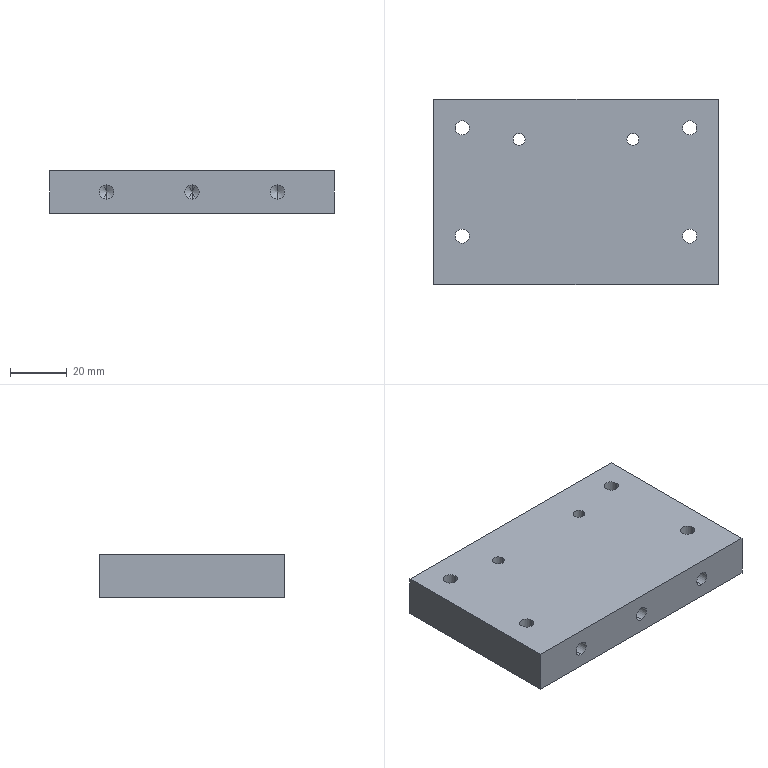Part | SolidWorks | features HoleWzd 4, Extrusion 1 | 1 solid | 46 faces | box 100 x 65 x 15 mm | volume 94078 mm3 | cylinder 24 | cone 16 | plane 6 | commonest cylinder face diameters 5 x20 4.2 x4
STEP:
#1=CARTESIAN_POINT('',(92.5,55.,15.));
#2=VERTEX_POINT('',#1);
#3=CARTESIAN_POINT('',(87.5,55.,15.));
#4=VERTEX_POINT('',#3);
#5=CARTESIAN_POINT('',(90.,55.,15.));
#6=DIRECTION('',(0.,0.,-1.));
#7=DIRECTION('',(-1.,0.,0.));
#8=AXIS2_PLACEMENT_3D('',#5,#6,#7);
#9=CIRCLE('',#8,2.5);
#10=EDGE_CURVE('',#2,#4,#9,.T.);
#11=ORIENTED_EDGE('',*,*,#10,.F.);
#12=CARTESIAN_POINT('',(92.5,55.,0.));
#13=VERTEX_POINT('',#12);
#14=CARTESIAN_POINT('',(92.5,55.,0.));
#15=DIRECTION('',(0.,0.,-1.));
#16=VECTOR('',#15,1000.);
#17=LINE('',#14,#16);
#18=EDGE_CURVE('',#2,#13,#17,.T.);
#19=ORIENTED_EDGE('',*,*,#18,.T.);
#20=CARTESIAN_POINT('',(87.5,55.,0.));
#21=VERTEX_POINT('',#20);
#22=CARTESIAN_POINT('',(90.,55.,0.));
#23=DIRECTION('',(0.,0.,-1.));
#24=DIRECTION('',(-1.,0.,0.));
#25=AXIS2_PLACEMENT_3D('',#22,#23,#24);
#26=CIRCLE('',#25,2.5);
#27=EDGE_CURVE('',#13,#21,#26,.T.);
#28=ORIENTED_EDGE('',*,*,#27,.T.);
#29=CARTESIAN_POINT('',(87.5,55.,0.));
#30=DIRECTION('',(0.,0.,-1.));
#31=VECTOR('',#30,1000.);
#32=LINE('',#29,#31);
#33=EDGE_CURVE('',#4,#21,#32,.T.);
#34=ORIENTED_EDGE('',*,*,#33,.F.);
#35=EDGE_LOOP('',(#11,#19,#28,#34));
#36=FACE_OUTER_BOUND('',#35,.T.);
#37=CARTESIAN_POINT('',(90.,55.,0.));
#38=DIRECTION('',(0.,0.,-1.));
#39=DIRECTION('',(-1.,0.,0.));
#40=AXIS2_PLACEMENT_3D('',#37,#38,#39);
#41=CYLINDRICAL_SURFACE('',#40,2.5);
#42=ADVANCED_FACE('',(#36),#41,.F.);
#43=CARTESIAN_POINT('',(12.5,55.,15.));
#44=VERTEX_POINT('',#43);
#45=CARTESIAN_POINT('',(7.5,55.,15.));
#46=VERTEX_POINT('',#45);
#47=CARTESIAN_POINT('',(10.,55.,15.));
#48=DIRECTION('',(0.,0.,-1.));
#49=DIRECTION('',(-1.,0.,0.));
#50=AXIS2_PLACEMENT_3D('',#47,#48,#49);
#51=CIRCLE('',#50,2.5);
#52=EDGE_CURVE('',#44,#46,#51,.T.);
#53=ORIENTED_EDGE('',*,*,#52,.F.);
#54=CARTESIAN_POINT('',(12.5,55.,0.));
#55=VERTEX_POINT('',#54);
#56=CARTESIAN_POINT('',(12.5,55.,0.));
#57=DIRECTION('',(0.,0.,-1.));
#58=VECTOR('',#57,1000.);
#59=LINE('',#56,#58);
#60=EDGE_CURVE('',#44,#55,#59,.T.);
#61=ORIENTED_EDGE('',*,*,#60,.T.);
#62=CARTESIAN_POINT('',(7.5,55.,0.));
#63=VERTEX_POINT('',#62);
#64=CARTESIAN_POINT('',(10.,55.,0.));
#65=DIRECTION('',(0.,0.,-1.));
#66=DIRECTION('',(-1.,0.,0.));
#67=AXIS2_PLACEMENT_3D('',#64,#65,#66);
#68=CIRCLE('',#67,2.5);
#69=EDGE_CURVE('',#55,#63,#68,.T.);
#70=ORIENTED_EDGE('',*,*,#69,.T.);
#71=CARTESIAN_POINT('',(7.5,55.,0.));
#72=DIRECTION('',(0.,0.,-1.));
#73=VECTOR('',#72,1000.);
#74=LINE('',#71,#73);
#75=EDGE_CURVE('',#46,#63,#74,.T.);
#76=ORIENTED_EDGE('',*,*,#75,.F.);
#77=EDGE_LOOP('',(#53,#61,#70,#76));
#78=FACE_OUTER_BOUND('',#77,.T.);
#79=CARTESIAN_POINT('',(10.,55.,0.));
#80=DIRECTION('',(0.,0.,-1.));
#81=DIRECTION('',(-1.,0.,0.));
#82=AXIS2_PLACEMENT_3D('',#79,#80,#81);
#83=CYLINDRICAL_SURFACE('',#82,2.5);
#84=ADVANCED_FACE('',(#78),#83,.F.);
#85=CARTESIAN_POINT('',(92.5,17.,15.));
#86=VERTEX_POINT('',#85);
#87=CARTESIAN_POINT('',(87.5,17.,15.));
#88=VERTEX_POINT('',#87);
#89=CARTESIAN_POINT('',(90.,17.,15.));
#90=DIRECTION('',(0.,0.,-1.));
#91=DIRECTION('',(-1.,0.,0.));
#92=AXIS2_PLACEMENT_3D('',#89,#90,#91);
#93=CIRCLE('',#92,2.5);
#94=EDGE_CURVE('',#86,#88,#93,.T.);
#95=ORIENTED_EDGE('',*,*,#94,.F.);
#96=CARTESIAN_POINT('',(92.5,17.,0.));
#97=VERTEX_POINT('',#96);
#98=CARTESIAN_POINT('',(92.5,17.,0.));
#99=DIRECTION('',(0.,0.,-1.));
#100=VECTOR('',#99,1000.);
#101=LINE('',#98,#100);
#102=EDGE_CURVE('',#86,#97,#101,.T.);
#103=ORIENTED_EDGE('',*,*,#102,.T.);
#104=CARTESIAN_POINT('',(87.5,17.,0.));
#105=VERTEX_POINT('',#104);
#106=CARTESIAN_POINT('',(90.,17.,0.));
#107=DIRECTION('',(0.,0.,-1.));
#108=DIRECTION('',(-1.,0.,0.));
#109=AXIS2_PLACEMENT_3D('',#106,#107,#108);
#110=CIRCLE('',#109,2.5);
#111=EDGE_CURVE('',#97,#105,#110,.T.);
#112=ORIENTED_EDGE('',*,*,#111,.T.);
#113=CARTESIAN_POINT('',(87.5,17.,0.));
#114=DIRECTION('',(0.,0.,-1.));
#115=VECTOR('',#114,1000.);
#116=LINE('',#113,#115);
#117=EDGE_CURVE('',#88,#105,#116,.T.);
#118=ORIENTED_EDGE('',*,*,#117,.F.);
#119=EDGE_LOOP('',(#95,#103,#112,#118));
#120=FACE_OUTER_BOUND('',#119,.T.);
#121=CARTESIAN_POINT('',(90.,17.,0.));
#122=DIRECTION('',(0.,0.,-1.));
#123=DIRECTION('',(-1.,0.,0.));
#124=AXIS2_PLACEMENT_3D('',#121,#122,#123);
#125=CYLINDRICAL_SURFACE('',#124,2.5);
#126=ADVANCED_FACE('',(#120),#125,.F.);
#127=CARTESIAN_POINT('',(12.5,17.,15.));
#128=VERTEX_POINT('',#127);
#129=CARTESIAN_POINT('',(7.5,17.,15.));
#130=VERTEX_POINT('',#129);
#131=CARTESIAN_POINT('',(10.,17.,15.));
#132=DIRECTION('',(0.,0.,-1.));
#133=DIRECTION('',(-1.,0.,0.));
#134=AXIS2_PLACEMENT_3D('',#131,#132,#133);
#135=CIRCLE('',#134,2.5);
#136=EDGE_CURVE('',#128,#130,#135,.T.);
#137=ORIENTED_EDGE('',*,*,#136,.F.);
#138=CARTESIAN_POINT('',(12.5,17.,0.));
#139=VERTEX_POINT('',#138);
#140=CARTESIAN_POINT('',(12.5,17.,0.));
#141=DIRECTION('',(0.,0.,-1.));
#142=VECTOR('',#141,1000.);
#143=LINE('',#140,#142);
#144=EDGE_CURVE('',#128,#139,#143,.T.);
#145=ORIENTED_EDGE('',*,*,#144,.T.);
#146=CARTESIAN_POINT('',(7.5,17.,0.));
#147=VERTEX_POINT('',#146);
#148=CARTESIAN_POINT('',(10.,17.,0.));
#149=DIRECTION('',(0.,0.,-1.));
#150=DIRECTION('',(-1.,0.,0.));
#151=AXIS2_PLACEMENT_3D('',#148,#149,#150);
#152=CIRCLE('',#151,2.5);
#153=EDGE_CURVE('',#139,#147,#152,.T.);
#154=ORIENTED_EDGE('',*,*,#153,.T.);
#155=CARTESIAN_POINT('',(7.5,17.,0.));
#156=DIRECTION('',(0.,0.,-1.));
#157=VECTOR('',#156,1000.);
#158=LINE('',#155,#157);
#159=EDGE_CURVE('',#130,#147,#158,.T.);
#160=ORIENTED_EDGE('',*,*,#159,.F.);
#161=EDGE_LOOP('',(#137,#145,#154,#160));
#162=FACE_OUTER_BOUND('',#161,.T.);
#163=CARTESIAN_POINT('',(10.,17.,0.));
#164=DIRECTION('',(0.,0.,-1.));
#165=DIRECTION('',(-1.,0.,0.));
#166=AXIS2_PLACEMENT_3D('',#163,#164,#165);
#167=CYLINDRICAL_SURFACE('',#166,2.5);
#168=ADVANCED_FACE('',(#162),#167,.F.);
#169=CARTESIAN_POINT('',(72.1,51.,0.425));
#170=VERTEX_POINT('',#169);
#171=CARTESIAN_POINT('',(67.9,51.,0.425));
#172=VERTEX_POINT('',#171);
#173=CARTESIAN_POINT('',(70.,51.,0.425));
#174=DIRECTION('',(0.,0.,-1.));
#175=DIRECTION('',(-1.,0.,0.));
#176=AXIS2_PLACEMENT_3D('',#173,#174,#175);
#177=CIRCLE('',#176,2.1);
#178=EDGE_CURVE('',#170,#172,#177,.T.);
#179=ORIENTED_EDGE('',*,*,#178,.F.);
#180=CARTESIAN_POINT('',(72.525,51.,0.));
#181=VERTEX_POINT('',#180);
#182=CARTESIAN_POINT('',(72.525,51.,0.));
#183=DIRECTION('',(0.7071,0.,-0.7071));
#184=VECTOR('',#183,1000.);
#185=LINE('',#182,#184);
#186=EDGE_CURVE('',#170,#181,#185,.T.);
#187=ORIENTED_EDGE('',*,*,#186,.T.);
#188=CARTESIAN_POINT('',(67.475,51.,0.));
#189=VERTEX_POINT('',#188);
#190=CARTESIAN_POINT('',(70.,51.,0.));
#191=DIRECTION('',(0.,0.,-1.));
#192=DIRECTION('',(-1.,0.,0.));
#193=AXIS2_PLACEMENT_3D('',#190,#191,#192);
#194=CIRCLE('',#193,2.525);
#195=EDGE_CURVE('',#181,#189,#194,.T.);
#196=ORIENTED_EDGE('',*,*,#195,.T.);
#197=CARTESIAN_POINT('',(67.475,51.,0.));
#198=DIRECTION('',(-0.7071,0.,-0.7071));
#199=VECTOR('',#198,1000.);
#200=LINE('',#197,#199);
#201=EDGE_CURVE('',#172,#189,#200,.T.);
#202=ORIENTED_EDGE('',*,*,#201,.F.);
#203=EDGE_LOOP('',(#179,#187,#196,#202));
#204=FACE_OUTER_BOUND('',#203,.T.);
#205=CARTESIAN_POINT('',(70.,51.,0.));
#206=DIRECTION('',(0.,0.,-1.));
#207=DIRECTION('',(-1.,0.,0.));
#208=AXIS2_PLACEMENT_3D('',#205,#206,#207);
#209=CONICAL_SURFACE('',#208,2.525,0.7854);
#210=ADVANCED_FACE('',(#204),#209,.F.);
#211=CARTESIAN_POINT('',(72.1,51.,15.));
#212=VERTEX_POINT('',#211);
#213=CARTESIAN_POINT('',(67.9,51.,15.));
#214=VERTEX_POINT('',#213);
#215=CARTESIAN_POINT('',(70.,51.,15.));
#216=DIRECTION('',(0.,0.,-1.));
#217=DIRECTION('',(-1.,0.,0.));
#218=AXIS2_PLACEMENT_3D('',#215,#216,#217);
#219=CIRCLE('',#218,2.1);
#220=EDGE_CURVE('',#212,#214,#219,.T.);
#221=ORIENTED_EDGE('',*,*,#220,.F.);
#222=CARTESIAN_POINT('',(72.1,51.,0.));
#223=DIRECTION('',(0.,0.,-1.));
#224=VECTOR('',#223,1000.);
#225=LINE('',#222,#224);
#226=EDGE_CURVE('',#212,#170,#225,.T.);
#227=ORIENTED_EDGE('',*,*,#226,.T.);
#228=ORIENTED_EDGE('',*,*,#178,.T.);
#229=CARTESIAN_POINT('',(67.9,51.,0.));
#230=DIRECTION('',(0.,0.,-1.));
#231=VECTOR('',#230,1000.);
#232=LINE('',#229,#231);
#233=EDGE_CURVE('',#214,#172,#232,.T.);
#234=ORIENTED_EDGE('',*,*,#233,.F.);
#235=EDGE_LOOP('',(#221,#227,#228,#234));
#236=FACE_OUTER_BOUND('',#235,.T.);
#237=CARTESIAN_POINT('',(70.,51.,0.));
#238=DIRECTION('',(0.,0.,-1.));
#239=DIRECTION('',(-1.,0.,0.));
#240=AXIS2_PLACEMENT_3D('',#237,#238,#239);
#241=CYLINDRICAL_SURFACE('',#240,2.1);
#242=ADVANCED_FACE('',(#236),#241,.F.);
#243=CARTESIAN_POINT('',(32.1,51.,0.425));
#244=VERTEX_POINT('',#243);
#245=CARTESIAN_POINT('',(27.9,51.,0.425));
#246=VERTEX_POINT('',#245);
#247=CARTESIAN_POINT('',(30.,51.,0.425));
#248=DIRECTION('',(0.,0.,-1.));
#249=DIRECTION('',(-1.,0.,0.));
#250=AXIS2_PLACEMENT_3D('',#247,#248,#249);
#251=CIRCLE('',#250,2.1);
#252=EDGE_CURVE('',#244,#246,#251,.T.);
#253=ORIENTED_EDGE('',*,*,#252,.F.);
#254=CARTESIAN_POINT('',(32.525,51.,0.));
#255=VERTEX_POINT('',#254);
#256=CARTESIAN_POINT('',(32.525,51.,0.));
#257=DIRECTION('',(0.7071,0.,-0.7071));
#258=VECTOR('',#257,1000.);
#259=LINE('',#256,#258);
#260=EDGE_CURVE('',#244,#255,#259,.T.);
#261=ORIENTED_EDGE('',*,*,#260,.T.);
#262=CARTESIAN_POINT('',(27.475,51.,0.));
#263=VERTEX_POINT('',#262);
#264=CARTESIAN_POINT('',(30.,51.,0.));
#265=DIRECTION('',(0.,0.,-1.));
#266=DIRECTION('',(-1.,0.,0.));
#267=AXIS2_PLACEMENT_3D('',#264,#265,#266);
#268=CIRCLE('',#267,2.525);
#269=EDGE_CURVE('',#255,#263,#268,.T.);
#270=ORIENTED_EDGE('',*,*,#269,.T.);
#271=CARTESIAN_POINT('',(27.475,51.,0.));
#272=DIRECTION('',(-0.7071,0.,-0.7071));
#273=VECTOR('',#272,1000.);
#274=LINE('',#271,#273);
#275=EDGE_CURVE('',#246,#263,#274,.T.);
#276=ORIENTED_EDGE('',*,*,#275,.F.);
#277=EDGE_LOOP('',(#253,#261,#270,#276));
#278=FACE_OUTER_BOUND('',#277,.T.);
#279=CARTESIAN_POINT('',(30.,51.,0.));
#280=DIRECTION('',(0.,0.,-1.));
#281=DIRECTION('',(-1.,0.,0.));
#282=AXIS2_PLACEMENT_3D('',#279,#280,#281);
#283=CONICAL_SURFACE('',#282,2.525,0.7854);
#284=ADVANCED_FACE('',(#278),#283,.F.);
#285=CARTESIAN_POINT('',(32.1,51.,15.));
#286=VERTEX_POINT('',#285);
#287=CARTESIAN_POINT('',(27.9,51.,15.));
#288=VERTEX_POINT('',#287);
#289=CARTESIAN_POINT('',(30.,51.,15.));
#290=DIRECTION('',(0.,0.,-1.));
#291=DIRECTION('',(-1.,0.,0.));
#292=AXIS2_PLACEMENT_3D('',#289,#290,#291);
#293=CIRCLE('',#292,2.1);
#294=EDGE_CURVE('',#286,#288,#293,.T.);
#295=ORIENTED_EDGE('',*,*,#294,.F.);
#296=CARTESIAN_POINT('',(32.1,51.,0.));
#297=DIRECTION('',(0.,0.,-1.));
#298=VECTOR('',#297,1000.);
#299=LINE('',#296,#298);
#300=EDGE_CURVE('',#286,#244,#299,.T.);
#301=ORIENTED_EDGE('',*,*,#300,.T.);
#302=ORIENTED_EDGE('',*,*,#252,.T.);
#303=CARTESIAN_POINT('',(27.9,51.,0.));
#304=DIRECTION('',(0.,0.,-1.));
#305=VECTOR('',#304,1000.);
#306=LINE('',#303,#305);
#307=EDGE_CURVE('',#288,#246,#306,.T.);
#308=ORIENTED_EDGE('',*,*,#307,.F.);
#309=EDGE_LOOP('',(#295,#301,#302,#308));
#310=FACE_OUTER_BOUND('',#309,.T.);
#311=CARTESIAN_POINT('',(30.,51.,0.));
#312=DIRECTION('',(0.,0.,-1.));
#313=DIRECTION('',(-1.,0.,0.));
#314=AXIS2_PLACEMENT_3D('',#311,#312,#313);
#315=CYLINDRICAL_SURFACE('',#314,2.1);
#316=ADVANCED_FACE('',(#310),#315,.F.);
#317=CARTESIAN_POINT('',(80.,15.,10.));
#318=VERTEX_POINT('',#317);
#319=CARTESIAN_POINT('',(80.,15.,5.));
#320=VERTEX_POINT('',#319);
#321=CARTESIAN_POINT('',(80.,15.,7.5));
#322=DIRECTION('',(0.,-1.,0.));
#323=DIRECTION('',(0.,0.,-1.));
#324=AXIS2_PLACEMENT_3D('',#321,#322,#323);
#325=CIRCLE('',#324,2.5);
#326=EDGE_CURVE('',#318,#320,#325,.T.);
#327=ORIENTED_EDGE('',*,*,#326,.F.);
#328=CARTESIAN_POINT('',(80.,0.,10.));
#329=VERTEX_POINT('',#328);
#330=CARTESIAN_POINT('',(80.,0.,10.));
#331=DIRECTION('',(0.,-1.,0.));
#332=VECTOR('',#331,1000.);
#333=LINE('',#330,#332);
#334=EDGE_CURVE('',#318,#329,#333,.T.);
#335=ORIENTED_EDGE('',*,*,#334,.T.);
#336=CARTESIAN_POINT('',(80.,0.,5.));
#337=VERTEX_POINT('',#336);
#338=CARTESIAN_POINT('',(80.,0.,7.5));
#339=DIRECTION('',(0.,-1.,0.));
#340=DIRECTION('',(0.,0.,-1.));
#341=AXIS2_PLACEMENT_3D('',#338,#339,#340);
#342=CIRCLE('',#341,2.5);
#343=EDGE_CURVE('',#329,#337,#342,.T.);
#344=ORIENTED_EDGE('',*,*,#343,.T.);
#345=CARTESIAN_POINT('',(80.,0.,5.));
#346=DIRECTION('',(0.,-1.,0.));
#347=VECTOR('',#346,1000.);
#348=LINE('',#345,#347);
#349=EDGE_CURVE('',#320,#337,#348,.T.);
#350=ORIENTED_EDGE('',*,*,#349,.F.);
#351=EDGE_LOOP('',(#327,#335,#344,#350));
#352=FACE_OUTER_BOUND('',#351,.T.);
#353=CARTESIAN_POINT('',(80.,0.,7.5));
#354=DIRECTION('',(0.,-1.,0.));
#355=DIRECTION('',(0.,0.,-1.));
#356=AXIS2_PLACEMENT_3D('',#353,#354,#355);
#357=CYLINDRICAL_SURFACE('',#356,2.5);
#358=ADVANCED_FACE('',(#352),#357,.F.);
#359=CARTESIAN_POINT('',(80.,16.502,7.5));
#360=VERTEX_POINT('',#359);
#361=CARTESIAN_POINT('',(80.,15.,5.));
#362=DIRECTION('',(0.,-0.515,-0.8572));
#363=VECTOR('',#362,1000.);
#364=LINE('',#361,#363);
#365=EDGE_CURVE('',#360,#320,#364,.T.);
#366=ORIENTED_EDGE('',*,*,#365,.F.);
#367=CARTESIAN_POINT('',(80.,15.,10.));
#368=DIRECTION('',(0.,-0.515,0.8572));
#369=VECTOR('',#368,1000.);
#370=LINE('',#367,#369);
#371=EDGE_CURVE('',#360,#318,#370,.T.);
#372=ORIENTED_EDGE('',*,*,#371,.T.);
#373=ORIENTED_EDGE('',*,*,#326,.T.);
#374=EDGE_LOOP('',(#366,#372,#373));
#375=FACE_OUTER_BOUND('',#374,.T.);
#376=CARTESIAN_POINT('',(80.,15.,7.5));
#377=DIRECTION('',(0.,-1.,0.));
#378=DIRECTION('',(0.,0.,-1.));
#379=AXIS2_PLACEMENT_3D('',#376,#377,#378);
#380=CONICAL_SURFACE('',#379,2.5,1.03);
#381=ADVANCED_FACE('',(#375),#380,.F.);
#382=CARTESIAN_POINT('',(50.,15.,10.));
#383=VERTEX_POINT('',#382);
#384=CARTESIAN_POINT('',(50.,15.,5.));
#385=VERTEX_POINT('',#384);
#386=CARTESIAN_POINT('',(50.,15.,7.5));
#387=DIRECTION('',(0.,-1.,0.));
#388=DIRECTION('',(0.,0.,-1.));
#389=AXIS2_PLACEMENT_3D('',#386,#387,#388);
#390=CIRCLE('',#389,2.5);
#391=EDGE_CURVE('',#383,#385,#390,.T.);
#392=ORIENTED_EDGE('',*,*,#391,.F.);
#393=CARTESIAN_POINT('',(50.,0.,10.));
#394=VERTEX_POINT('',#393);
#395=CARTESIAN_POINT('',(50.,0.,10.));
#396=DIRECTION('',(0.,-1.,0.));
#397=VECTOR('',#396,1000.);
#398=LINE('',#395,#397);
#399=EDGE_CURVE('',#383,#394,#398,.T.);
#400=ORIENTED_EDGE('',*,*,#399,.T.);
#401=CARTESIAN_POINT('',(50.,0.,5.));
#402=VERTEX_POINT('',#401);
#403=CARTESIAN_POINT('',(50.,0.,7.5));
#404=DIRECTION('',(0.,-1.,0.));
#405=DIRECTION('',(0.,0.,-1.));
#406=AXIS2_PLACEMENT_3D('',#403,#404,#405);
#407=CIRCLE('',#406,2.5);
#408=EDGE_CURVE('',#394,#402,#407,.T.);
#409=ORIENTED_EDGE('',*,*,#408,.T.);
#410=CARTESIAN_POINT('',(50.,0.,5.));
#411=DIRECTION('',(0.,-1.,0.));
#412=VECTOR('',#411,1000.);
#413=LINE('',#410,#412);
#414=EDGE_CURVE('',#385,#402,#413,.T.);
#415=ORIENTED_EDGE('',*,*,#414,.F.);
#416=EDGE_LOOP('',(#392,#400,#409,#415));
#417=FACE_OUTER_BOUND('',#416,.T.);
#418=CARTESIAN_POINT('',(50.,0.,7.5));
#419=DIRECTION('',(0.,-1.,0.));
#420=DIRECTION('',(0.,0.,-1.));
#421=AXIS2_PLACEMENT_3D('',#418,#419,#420);
#422=CYLINDRICAL_SURFACE('',#421,2.5);
#423=ADVANCED_FACE('',(#417),#422,.F.);
#424=CARTESIAN_POINT('',(50.,16.502,7.5));
#425=VERTEX_POINT('',#424);
#426=CARTESIAN_POINT('',(50.,15.,5.));
#427=DIRECTION('',(0.,-0.515,-0.8572));
#428=VECTOR('',#427,1000.);
#429=LINE('',#426,#428);
#430=EDGE_CURVE('',#425,#385,#429,.T.);
#431=ORIENTED_EDGE('',*,*,#430,.F.);
#432=CARTESIAN_POINT('',(50.,15.,10.));
#433=DIRECTION('',(0.,-0.515,0.8572));
#434=VECTOR('',#433,1000.);
#435=LINE('',#432,#434);
#436=EDGE_CURVE('',#425,#383,#435,.T.);
#437=ORIENTED_EDGE('',*,*,#436,.T.);
#438=ORIENTED_EDGE('',*,*,#391,.T.);
#439=EDGE_LOOP('',(#431,#437,#438));
#440=FACE_OUTER_BOUND('',#439,.T.);
#441=CARTESIAN_POINT('',(50.,15.,7.5));
#442=DIRECTION('',(0.,-1.,0.));
#443=DIRECTION('',(0.,0.,-1.));
#444=AXIS2_PLACEMENT_3D('',#441,#442,#443);
#445=CONICAL_SURFACE('',#444,2.5,1.03);
#446=ADVANCED_FACE('',(#440),#445,.F.);
#447=CARTESIAN_POINT('',(20.,15.,10.));
#448=VERTEX_POINT('',#447);
#449=CARTESIAN_POINT('',(20.,15.,5.));
#450=VERTEX_POINT('',#449);
#451=CARTESIAN_POINT('',(20.,15.,7.5));
#452=DIRECTION('',(0.,-1.,0.));
#453=DIRECTION('',(0.,0.,-1.));
#454=AXIS2_PLACEMENT_3D('',#451,#452,#453);
#455=CIRCLE('',#454,2.5);
#456=EDGE_CURVE('',#448,#450,#455,.T.);
#457=ORIENTED_EDGE('',*,*,#456,.F.);
#458=CARTESIAN_POINT('',(20.,0.,10.));
#459=VERTEX_POINT('',#458);
#460=CARTESIAN_POINT('',(20.,0.,10.));
#461=DIRECTION('',(0.,-1.,0.));
#462=VECTOR('',#461,1000.);
#463=LINE('',#460,#462);
#464=EDGE_CURVE('',#448,#459,#463,.T.);
#465=ORIENTED_EDGE('',*,*,#464,.T.);
#466=CARTESIAN_POINT('',(20.,0.,5.));
#467=VERTEX_POINT('',#466);
#468=CARTESIAN_POINT('',(20.,0.,7.5));
#469=DIRECTION('',(0.,-1.,0.));
#470=DIRECTION('',(0.,0.,-1.));
#471=AXIS2_PLACEMENT_3D('',#468,#469,#470);
#472=CIRCLE('',#471,2.5);
#473=EDGE_CURVE('',#459,#467,#472,.T.);
#474=ORIENTED_EDGE('',*,*,#473,.T.);
#475=CARTESIAN_POINT('',(20.,0.,5.));
#476=DIRECTION('',(0.,-1.,0.));
#477=VECTOR('',#476,1000.);
#478=LINE('',#475,#477);
#479=EDGE_CURVE('',#450,#467,#478,.T.);
#480=ORIENTED_EDGE('',*,*,#479,.F.);
#481=EDGE_LOOP('',(#457,#465,#474,#480));
#482=FACE_OUTER_BOUND('',#481,.T.);
#483=CARTESIAN_POINT('',(20.,0.,7.5));
#484=DIRECTION('',(0.,-1.,0.));
#485=DIRECTION('',(0.,0.,-1.));
#486=AXIS2_PLACEMENT_3D('',#483,#484,#485);
#487=CYLINDRICAL_SURFACE('',#486,2.5);
#488=ADVANCED_FACE('',(#482),#487,.F.);
#489=CARTESIAN_POINT('',(20.,16.502,7.5));
#490=VERTEX_POINT('',#489);
#491=CARTESIAN_POINT('',(20.,15.,5.));
#492=DIRECTION('',(0.,-0.515,-0.8572));
#493=VECTOR('',#492,1000.);
#494=LINE('',#491,#493);
#495=EDGE_CURVE('',#490,#450,#494,.T.);
#496=ORIENTED_EDGE('',*,*,#495,.F.);
#497=CARTESIAN_POINT('',(20.,15.,10.));
#498=DIRECTION('',(0.,-0.515,0.8572));
#499=VECTOR('',#498,1000.);
#500=LINE('',#497,#499);
#501=EDGE_CURVE('',#490,#448,#500,.T.);
#502=ORIENTED_EDGE('',*,*,#501,.T.);
#503=ORIENTED_EDGE('',*,*,#456,.T.);
#504=EDGE_LOOP('',(#496,#502,#503));
#505=FACE_OUTER_BOUND('',#504,.T.);
#506=CARTESIAN_POINT('',(20.,15.,7.5));
#507=DIRECTION('',(0.,-1.,0.));
#508=DIRECTION('',(0.,0.,-1.));
#509=AXIS2_PLACEMENT_3D('',#506,#507,#508);
#510=CONICAL_SURFACE('',#509,2.5,1.03);
#511=ADVANCED_FACE('',(#505),#510,.F.);
#512=CARTESIAN_POINT('',(20.,50.,5.));
#513=VERTEX_POINT('',#512);
#514=CARTESIAN_POINT('',(20.,50.,10.));
#515=VERTEX_POINT('',#514);
#516=CARTESIAN_POINT('',(20.,50.,7.5));
#517=DIRECTION('',(0.,1.,0.));
#518=DIRECTION('',(0.,0.,1.));
#519=AXIS2_PLACEMENT_3D('',#516,#517,#518);
#520=CIRCLE('',#519,2.5);
#521=EDGE_CURVE('',#513,#515,#520,.T.);
#522=ORIENTED_EDGE('',*,*,#521,.F.);
#523=CARTESIAN_POINT('',(20.,65.,5.));
#524=VERTEX_POINT('',#523);
#525=CARTESIAN_POINT('',(20.,65.,5.));
#526=DIRECTION('',(0.,1.,0.));
#527=VECTOR('',#526,1000.);
#528=LINE('',#525,#527);
#529=EDGE_CURVE('',#513,#524,#528,.T.);
#530=ORIENTED_EDGE('',*,*,#529,.T.);
#531=CARTESIAN_POINT('',(20.,65.,10.));
#532=VERTEX_POINT('',#531);
#533=CARTESIAN_POINT('',(20.,65.,7.5));
#534=DIRECTION('',(0.,1.,0.));
#535=DIRECTION('',(0.,0.,1.));
#536=AXIS2_PLACEMENT_3D('',#533,#534,#535);
#537=CIRCLE('',#536,2.5);
#538=EDGE_CURVE('',#524,#532,#537,.T.);
#539=ORIENTED_EDGE('',*,*,#538,.T.);
#540=CARTESIAN_POINT('',(20.,65.,10.));
#541=DIRECTION('',(0.,1.,0.));
#542=VECTOR('',#541,1000.);
#543=LINE('',#540,#542);
#544=EDGE_CURVE('',#515,#532,#543,.T.);
#545=ORIENTED_EDGE('',*,*,#544,.F.);
#546=EDGE_LOOP('',(#522,#530,#539,#545));
#547=FACE_OUTER_BOUND('',#546,.T.);
#548=CARTESIAN_POINT('',(20.,65.,7.5));
#549=DIRECTION('',(0.,1.,0.));
#550=DIRECTION('',(0.,0.,1.));
#551=AXIS2_PLACEMENT_3D('',#548,#549,#550);
#552=CYLINDRICAL_SURFACE('',#551,2.5);
#553=ADVANCED_FACE('',(#547),#552,.F.);
#554=CARTESIAN_POINT('',(20.,48.498,7.5));
#555=VERTEX_POINT('',#554);
#556=CARTESIAN_POINT('',(20.,50.,10.));
#557=DIRECTION('',(0.,0.515,0.8572));
#558=VECTOR('',#557,1000.);
#559=LINE('',#556,#558);
#560=EDGE_CURVE('',#555,#515,#559,.T.);
#561=ORIENTED_EDGE('',*,*,#560,.F.);
#562=CARTESIAN_POINT('',(20.,50.,5.));
#563=DIRECTION('',(0.,0.515,-0.8572));
#564=VECTOR('',#563,1000.);
#565=LINE('',#562,#564);
#566=EDGE_CURVE('',#555,#513,#565,.T.);
#567=ORIENTED_EDGE('',*,*,#566,.T.);
#568=ORIENTED_EDGE('',*,*,#521,.T.);
#569=EDGE_LOOP('',(#561,#567,#568));
#570=FACE_OUTER_BOUND('',#569,.T.);
#571=CARTESIAN_POINT('',(20.,50.,7.5));
#572=DIRECTION('',(0.,1.,0.));
#573=DIRECTION('',(0.,0.,1.));
#574=AXIS2_PLACEMENT_3D('',#571,#572,#573);
#575=CONICAL_SURFACE('',#574,2.5,1.03);
#576=ADVANCED_FACE('',(#570),#575,.F.);
#577=CARTESIAN_POINT('',(80.,50.,5.));
#578=VERTEX_POINT('',#577);
#579=CARTESIAN_POINT('',(80.,50.,10.));
#580=VERTEX_POINT('',#579);
#581=CARTESIAN_POINT('',(80.,50.,7.5));
#582=DIRECTION('',(0.,1.,0.));
#583=DIRECTION('',(0.,0.,1.));
#584=AXIS2_PLACEMENT_3D('',#581,#582,#583);
#585=CIRCLE('',#584,2.5);
#586=EDGE_CURVE('',#578,#580,#585,.T.);
#587=ORIENTED_EDGE('',*,*,#586,.F.);
#588=CARTESIAN_POINT('',(80.,65.,5.));
#589=VERTEX_POINT('',#588);
#590=CARTESIAN_POINT('',(80.,65.,5.));
#591=DIRECTION('',(0.,1.,0.));
#592=VECTOR('',#591,1000.);
#593=LINE('',#590,#592);
#594=EDGE_CURVE('',#578,#589,#593,.T.);
#595=ORIENTED_EDGE('',*,*,#594,.T.);
#596=CARTESIAN_POINT('',(80.,65.,10.));
#597=VERTEX_POINT('',#596);
#598=CARTESIAN_POINT('',(80.,65.,7.5));
#599=DIRECTION('',(0.,1.,0.));
#600=DIRECTION('',(0.,0.,1.));
#601=AXIS2_PLACEMENT_3D('',#598,#599,#600);
#602=CIRCLE('',#601,2.5);
#603=EDGE_CURVE('',#589,#597,#602,.T.);
#604=ORIENTED_EDGE('',*,*,#603,.T.);
#605=CARTESIAN_POINT('',(80.,65.,10.));
#606=DIRECTION('',(0.,1.,0.));
#607=VECTOR('',#606,1000.);
#608=LINE('',#605,#607);
#609=EDGE_CURVE('',#580,#597,#608,.T.);
#610=ORIENTED_EDGE('',*,*,#609,.F.);
#611=EDGE_LOOP('',(#587,#595,#604,#610));
#612=FACE_OUTER_BOUND('',#611,.T.);
#613=CARTESIAN_POINT('',(80.,65.,7.5));
#614=DIRECTION('',(0.,1.,0.));
#615=DIRECTION('',(0.,0.,1.));
#616=AXIS2_PLACEMENT_3D('',#613,#614,#615);
#617=CYLINDRICAL_SURFACE('',#616,2.5);
#618=ADVANCED_FACE('',(#612),#617,.F.);
#619=CARTESIAN_POINT('',(80.,48.498,7.5));
#620=VERTEX_POINT('',#619);
#621=CARTESIAN_POINT('',(80.,50.,10.));
#622=DIRECTION('',(0.,0.515,0.8572));
#623=VECTOR('',#622,1000.);
#624=LINE('',#621,#623);
#625=EDGE_CURVE('',#620,#580,#624,.T.);
#626=ORIENTED_EDGE('',*,*,#625,.F.);
#627=CARTESIAN_POINT('',(80.,50.,5.));
#628=DIRECTION('',(0.,0.515,-0.8572));
#629=VECTOR('',#628,1000.);
#630=LINE('',#627,#629);
#631=EDGE_CURVE('',#620,#578,#630,.T.);
#632=ORIENTED_EDGE('',*,*,#631,.T.);
#633=ORIENTED_EDGE('',*,*,#586,.T.);
#634=EDGE_LOOP('',(#626,#632,#633));
#635=FACE_OUTER_BOUND('',#634,.T.);
#636=CARTESIAN_POINT('',(80.,50.,7.5));
#637=DIRECTION('',(0.,1.,0.));
#638=DIRECTION('',(0.,0.,1.));
#639=AXIS2_PLACEMENT_3D('',#636,#637,#638);
#640=CONICAL_SURFACE('',#639,2.5,1.03);
#641=ADVANCED_FACE('',(#635),#640,.F.);
#642=CARTESIAN_POINT('',(50.,50.,5.));
#643=VERTEX_POINT('',#642);
#644=CARTESIAN_POINT('',(50.,50.,10.));
#645=VERTEX_POINT('',#644);
#646=CARTESIAN_POINT('',(50.,50.,7.5));
#647=DIRECTION('',(0.,1.,0.));
#648=DIRECTION('',(0.,0.,1.));
#649=AXIS2_PLACEMENT_3D('',#646,#647,#648);
#650=CIRCLE('',#649,2.5);
#651=EDGE_CURVE('',#643,#645,#650,.T.);
#652=ORIENTED_EDGE('',*,*,#651,.F.);
#653=CARTESIAN_POINT('',(50.,65.,5.));
#654=VERTEX_POINT('',#653);
#655=CARTESIAN_POINT('',(50.,65.,5.));
#656=DIRECTION('',(0.,1.,0.));
#657=VECTOR('',#656,1000.);
#658=LINE('',#655,#657);
#659=EDGE_CURVE('',#643,#654,#658,.T.);
#660=ORIENTED_EDGE('',*,*,#659,.T.);
#661=CARTESIAN_POINT('',(50.,65.,10.));
#662=VERTEX_POINT('',#661);
#663=CARTESIAN_POINT('',(50.,65.,7.5));
#664=DIRECTION('',(0.,1.,0.));
#665=DIRECTION('',(0.,0.,1.));
#666=AXIS2_PLACEMENT_3D('',#663,#664,#665);
#667=CIRCLE('',#666,2.5);
#668=EDGE_CURVE('',#654,#662,#667,.T.);
#669=ORIENTED_EDGE('',*,*,#668,.T.);
#670=CARTESIAN_POINT('',(50.,65.,10.));
#671=DIRECTION('',(0.,1.,0.));
#672=VECTOR('',#671,1000.);
#673=LINE('',#670,#672);
#674=EDGE_CURVE('',#645,#662,#673,.T.);
#675=ORIENTED_EDGE('',*,*,#674,.F.);
#676=EDGE_LOOP('',(#652,#660,#669,#675));
#677=FACE_OUTER_BOUND('',#676,.T.);
#678=CARTESIAN_POINT('',(50.,65.,7.5));
#679=DIRECTION('',(0.,1.,0.));
#680=DIRECTION('',(0.,0.,1.));
#681=AXIS2_PLACEMENT_3D('',#678,#679,#680);
#682=CYLINDRICAL_SURFACE('',#681,2.5);
#683=ADVANCED_FACE('',(#677),#682,.F.);
#684=CARTESIAN_POINT('',(50.,48.498,7.5));
#685=VERTEX_POINT('',#684);
#686=CARTESIAN_POINT('',(50.,50.,10.));
#687=DIRECTION('',(0.,0.515,0.8572));
#688=VECTOR('',#687,1000.);
#689=LINE('',#686,#688);
#690=EDGE_CURVE('',#685,#645,#689,.T.);
#691=ORIENTED_EDGE('',*,*,#690,.F.);
#692=CARTESIAN_POINT('',(50.,50.,5.));
#693=DIRECTION('',(0.,0.515,-0.8572));
#694=VECTOR('',#693,1000.);
#695=LINE('',#692,#694);
#696=EDGE_CURVE('',#685,#643,#695,.T.);
#697=ORIENTED_EDGE('',*,*,#696,.T.);
#698=ORIENTED_EDGE('',*,*,#651,.T.);
#699=EDGE_LOOP('',(#691,#697,#698));
#700=FACE_OUTER_BOUND('',#699,.T.);
#701=CARTESIAN_POINT('',(50.,50.,7.5));
#702=DIRECTION('',(0.,1.,0.));
#703=DIRECTION('',(0.,0.,1.));
#704=AXIS2_PLACEMENT_3D('',#701,#702,#703);
#705=CONICAL_SURFACE('',#704,2.5,1.03);
#706=ADVANCED_FACE('',(#700),#705,.F.);
#707=CARTESIAN_POINT('',(0.,65.,0.));
#708=VERTEX_POINT('',#707);
#709=CARTESIAN_POINT('',(0.,0.,0.));
#710=VERTEX_POINT('',#709);
#711=CARTESIAN_POINT('',(0.,0.,0.));
#712=DIRECTION('',(0.,-1.,0.));
#713=VECTOR('',#712,1000.);
#714=LINE('',#711,#713);
#715=EDGE_CURVE('',#708,#710,#714,.T.);
#716=ORIENTED_EDGE('',*,*,#715,.T.);
#717=CARTESIAN_POINT('',(0.,0.,15.));
#718=VERTEX_POINT('',#717);
#719=CARTESIAN_POINT('',(0.,0.,15.));
#720=DIRECTION('',(0.,0.,-1.));
#721=VECTOR('',#720,1000.);
#722=LINE('',#719,#721);
#723=EDGE_CURVE('',#718,#710,#722,.T.);
#724=ORIENTED_EDGE('',*,*,#723,.F.);
#725=CARTESIAN_POINT('',(0.,65.,15.));
#726=VERTEX_POINT('',#725);
#727=CARTESIAN_POINT('',(0.,0.,15.));
#728=DIRECTION('',(0.,-1.,0.));
#729=VECTOR('',#728,1000.);
#730=LINE('',#727,#729);
#731=EDGE_CURVE('',#726,#718,#730,.T.);
#732=ORIENTED_EDGE('',*,*,#731,.F.);
#733=CARTESIAN_POINT('',(0.,65.,15.));
#734=DIRECTION('',(0.,0.,-1.));
#735=VECTOR('',#734,1000.);
#736=LINE('',#733,#735);
#737=EDGE_CURVE('',#726,#708,#736,.T.);
#738=ORIENTED_EDGE('',*,*,#737,.T.);
#739=EDGE_LOOP('',(#716,#724,#732,#738));
#740=FACE_OUTER_BOUND('',#739,.T.);
#741=CARTESIAN_POINT('',(0.,0.,15.));
#742=DIRECTION('',(1.,0.,0.));
#743=DIRECTION('',(0.,1.,0.));
#744=AXIS2_PLACEMENT_3D('',#741,#742,#743);
#745=PLANE('',#744);
#746=ADVANCED_FACE('',(#740),#745,.F.);
#747=CARTESIAN_POINT('',(80.,0.,7.5));
#748=DIRECTION('',(0.,-1.,0.));
#749=DIRECTION('',(0.,0.,-1.));
#750=AXIS2_PLACEMENT_3D('',#747,#748,#749);
#751=CIRCLE('',#750,2.5);
#752=EDGE_CURVE('',#337,#329,#751,.T.);
#753=ORIENTED_EDGE('',*,*,#752,.F.);
#754=ORIENTED_EDGE('',*,*,#343,.F.);
#755=EDGE_LOOP('',(#753,#754));
#756=FACE_BOUND('',#755,.T.);
#757=CARTESIAN_POINT('',(50.,0.,7.5));
#758=DIRECTION('',(0.,-1.,0.));
#759=DIRECTION('',(0.,0.,-1.));
#760=AXIS2_PLACEMENT_3D('',#757,#758,#759);
#761=CIRCLE('',#760,2.5);
#762=EDGE_CURVE('',#402,#394,#761,.T.);
#763=ORIENTED_EDGE('',*,*,#762,.F.);
#764=ORIENTED_EDGE('',*,*,#408,.F.);
#765=EDGE_LOOP('',(#763,#764));
#766=FACE_BOUND('',#765,.T.);
#767=CARTESIAN_POINT('',(20.,0.,7.5));
#768=DIRECTION('',(0.,-1.,0.));
#769=DIRECTION('',(0.,0.,-1.));
#770=AXIS2_PLACEMENT_3D('',#767,#768,#769);
#771=CIRCLE('',#770,2.5);
#772=EDGE_CURVE('',#467,#459,#771,.T.);
#773=ORIENTED_EDGE('',*,*,#772,.F.);
#774=ORIENTED_EDGE('',*,*,#473,.F.);
#775=EDGE_LOOP('',(#773,#774));
#776=FACE_BOUND('',#775,.T.);
#777=CARTESIAN_POINT('',(100.,0.,0.));
#778=VERTEX_POINT('',#777);
#779=CARTESIAN_POINT('',(0.,0.,0.));
#780=DIRECTION('',(1.,0.,0.));
#781=VECTOR('',#780,1000.);
#782=LINE('',#779,#781);
#783=EDGE_CURVE('',#710,#778,#782,.T.);
#784=ORIENTED_EDGE('',*,*,#783,.T.);
#785=CARTESIAN_POINT('',(100.,0.,15.));
#786=VERTEX_POINT('',#785);
#787=CARTESIAN_POINT('',(100.,0.,15.));
#788=DIRECTION('',(0.,0.,-1.));
#789=VECTOR('',#788,1000.);
#790=LINE('',#787,#789);
#791=EDGE_CURVE('',#786,#778,#790,.T.);
#792=ORIENTED_EDGE('',*,*,#791,.F.);
#793=CARTESIAN_POINT('',(0.,0.,15.));
#794=DIRECTION('',(1.,0.,0.));
#795=VECTOR('',#794,1000.);
#796=LINE('',#793,#795);
#797=EDGE_CURVE('',#718,#786,#796,.T.);
#798=ORIENTED_EDGE('',*,*,#797,.F.);
#799=ORIENTED_EDGE('',*,*,#723,.T.);
#800=EDGE_LOOP('',(#784,#792,#798,#799));
#801=FACE_OUTER_BOUND('',#800,.T.);
#802=CARTESIAN_POINT('',(0.,0.,15.));
#803=DIRECTION('',(0.,1.,0.));
#804=DIRECTION('',(0.,0.,1.));
#805=AXIS2_PLACEMENT_3D('',#802,#803,#804);
#806=PLANE('',#805);
#807=ADVANCED_FACE('',(#756,#766,#776,#801),#806,.F.);
#808=CARTESIAN_POINT('',(100.,65.,0.));
#809=VERTEX_POINT('',#808);
#810=CARTESIAN_POINT('',(100.,0.,0.));
#811=DIRECTION('',(0.,1.,0.));
#812=VECTOR('',#811,1000.);
#813=LINE('',#810,#812);
#814=EDGE_CURVE('',#778,#809,#813,.T.);
#815=ORIENTED_EDGE('',*,*,#814,.T.);
#816=CARTESIAN_POINT('',(100.,65.,15.));
#817=VERTEX_POINT('',#816);
#818=CARTESIAN_POINT('',(100.,65.,15.));
#819=DIRECTION('',(0.,0.,-1.));
#820=VECTOR('',#819,1000.);
#821=LINE('',#818,#820);
#822=EDGE_CURVE('',#817,#809,#821,.T.);
#823=ORIENTED_EDGE('',*,*,#822,.F.);
#824=CARTESIAN_POINT('',(100.,0.,15.));
#825=DIRECTION('',(0.,1.,0.));
#826=VECTOR('',#825,1000.);
#827=LINE('',#824,#826);
#828=EDGE_CURVE('',#786,#817,#827,.T.);
#829=ORIENTED_EDGE('',*,*,#828,.F.);
#830=ORIENTED_EDGE('',*,*,#791,.T.);
#831=EDGE_LOOP('',(#815,#823,#829,#830));
#832=FACE_OUTER_BOUND('',#831,.T.);
#833=CARTESIAN_POINT('',(100.,0.,15.));
#834=DIRECTION('',(-1.,0.,0.));
#835=DIRECTION('',(0.,-1.,0.));
#836=AXIS2_PLACEMENT_3D('',#833,#834,#835);
#837=PLANE('',#836);
#838=ADVANCED_FACE('',(#832),#837,.F.);
#839=CARTESIAN_POINT('',(20.,65.,7.5));
#840=DIRECTION('',(0.,1.,0.));
#841=DIRECTION('',(0.,0.,1.));
#842=AXIS2_PLACEMENT_3D('',#839,#840,#841);
#843=CIRCLE('',#842,2.5);
#844=EDGE_CURVE('',#532,#524,#843,.T.);
#845=ORIENTED_EDGE('',*,*,#844,.F.);
#846=ORIENTED_EDGE('',*,*,#538,.F.);
#847=EDGE_LOOP('',(#845,#846));
#848=FACE_BOUND('',#847,.T.);
#849=CARTESIAN_POINT('',(80.,65.,7.5));
#850=DIRECTION('',(0.,1.,0.));
#851=DIRECTION('',(0.,0.,1.));
#852=AXIS2_PLACEMENT_3D('',#849,#850,#851);
#853=CIRCLE('',#852,2.5);
#854=EDGE_CURVE('',#597,#589,#853,.T.);
#855=ORIENTED_EDGE('',*,*,#854,.F.);
#856=ORIENTED_EDGE('',*,*,#603,.F.);
#857=EDGE_LOOP('',(#855,#856));
#858=FACE_BOUND('',#857,.T.);
#859=CARTESIAN_POINT('',(50.,65.,7.5));
#860=DIRECTION('',(0.,1.,0.));
#861=DIRECTION('',(0.,0.,1.));
#862=AXIS2_PLACEMENT_3D('',#859,#860,#861);
#863=CIRCLE('',#862,2.5);
#864=EDGE_CURVE('',#662,#654,#863,.T.);
#865=ORIENTED_EDGE('',*,*,#864,.F.);
#866=ORIENTED_EDGE('',*,*,#668,.F.);
#867=EDGE_LOOP('',(#865,#866));
#868=FACE_BOUND('',#867,.T.);
#869=CARTESIAN_POINT('',(0.,65.,0.));
#870=DIRECTION('',(-1.,0.,0.));
#871=VECTOR('',#870,1000.);
#872=LINE('',#869,#871);
#873=EDGE_CURVE('',#809,#708,#872,.T.);
#874=ORIENTED_EDGE('',*,*,#873,.T.);
#875=ORIENTED_EDGE('',*,*,#737,.F.);
#876=CARTESIAN_POINT('',(0.,65.,15.));
#877=DIRECTION('',(-1.,0.,0.));
#878=VECTOR('',#877,1000.);
#879=LINE('',#876,#878);
#880=EDGE_CURVE('',#817,#726,#879,.T.);
#881=ORIENTED_EDGE('',*,*,#880,.F.);
#882=ORIENTED_EDGE('',*,*,#822,.T.);
#883=EDGE_LOOP('',(#874,#875,#881,#882));
#884=FACE_OUTER_BOUND('',#883,.T.);
#885=CARTESIAN_POINT('',(0.,65.,15.));
#886=DIRECTION('',(0.,-1.,0.));
#887=DIRECTION('',(0.,0.,-1.));
#888=AXIS2_PLACEMENT_3D('',#885,#886,#887);
#889=PLANE('',#888);
#890=ADVANCED_FACE('',(#848,#858,#868,#884),#889,.F.);
#891=CARTESIAN_POINT('',(90.,55.,15.));
#892=DIRECTION('',(0.,0.,-1.));
#893=DIRECTION('',(-1.,0.,0.));
#894=AXIS2_PLACEMENT_3D('',#891,#892,#893);
#895=CIRCLE('',#894,2.5);
#896=EDGE_CURVE('',#4,#2,#895,.T.);
#897=ORIENTED_EDGE('',*,*,#896,.T.);
#898=ORIENTED_EDGE('',*,*,#10,.T.);
#899=EDGE_LOOP('',(#897,#898));
#900=FACE_BOUND('',#899,.T.);
#901=CARTESIAN_POINT('',(10.,55.,15.));
#902=DIRECTION('',(0.,0.,-1.));
#903=DIRECTION('',(-1.,0.,0.));
#904=AXIS2_PLACEMENT_3D('',#901,#902,#903);
#905=CIRCLE('',#904,2.5);
#906=EDGE_CURVE('',#46,#44,#905,.T.);
#907=ORIENTED_EDGE('',*,*,#906,.T.);
#908=ORIENTED_EDGE('',*,*,#52,.T.);
#909=EDGE_LOOP('',(#907,#908));
#910=FACE_BOUND('',#909,.T.);
#911=CARTESIAN_POINT('',(90.,17.,15.));
#912=DIRECTION('',(0.,0.,-1.));
#913=DIRECTION('',(-1.,0.,0.));
#914=AXIS2_PLACEMENT_3D('',#911,#912,#913);
#915=CIRCLE('',#914,2.5);
#916=EDGE_CURVE('',#88,#86,#915,.T.);
#917=ORIENTED_EDGE('',*,*,#916,.T.);
#918=ORIENTED_EDGE('',*,*,#94,.T.);
#919=EDGE_LOOP('',(#917,#918));
#920=FACE_BOUND('',#919,.T.);
#921=CARTESIAN_POINT('',(10.,17.,15.));
#922=DIRECTION('',(0.,0.,-1.));
#923=DIRECTION('',(-1.,0.,0.));
#924=AXIS2_PLACEMENT_3D('',#921,#922,#923);
#925=CIRCLE('',#924,2.5);
#926=EDGE_CURVE('',#130,#128,#925,.T.);
#927=ORIENTED_EDGE('',*,*,#926,.T.);
#928=ORIENTED_EDGE('',*,*,#136,.T.);
#929=EDGE_LOOP('',(#927,#928));
#930=FACE_BOUND('',#929,.T.);
#931=CARTESIAN_POINT('',(70.,51.,15.));
#932=DIRECTION('',(0.,0.,-1.));
#933=DIRECTION('',(-1.,0.,0.));
#934=AXIS2_PLACEMENT_3D('',#931,#932,#933);
#935=CIRCLE('',#934,2.1);
#936=EDGE_CURVE('',#214,#212,#935,.T.);
#937=ORIENTED_EDGE('',*,*,#936,.T.);
#938=ORIENTED_EDGE('',*,*,#220,.T.);
#939=EDGE_LOOP('',(#937,#938));
#940=FACE_BOUND('',#939,.T.);
#941=CARTESIAN_POINT('',(30.,51.,15.));
#942=DIRECTION('',(0.,0.,-1.));
#943=DIRECTION('',(-1.,0.,0.));
#944=AXIS2_PLACEMENT_3D('',#941,#942,#943);
#945=CIRCLE('',#944,2.1);
#946=EDGE_CURVE('',#288,#286,#945,.T.);
#947=ORIENTED_EDGE('',*,*,#946,.T.);
#948=ORIENTED_EDGE('',*,*,#294,.T.);
#949=EDGE_LOOP('',(#947,#948));
#950=FACE_BOUND('',#949,.T.);
#951=ORIENTED_EDGE('',*,*,#731,.T.);
#952=ORIENTED_EDGE('',*,*,#797,.T.);
#953=ORIENTED_EDGE('',*,*,#828,.T.);
#954=ORIENTED_EDGE('',*,*,#880,.T.);
#955=EDGE_LOOP('',(#951,#952,#953,#954));
#956=FACE_OUTER_BOUND('',#955,.T.);
#957=CARTESIAN_POINT('',(0.,0.,15.));
#958=DIRECTION('',(0.,0.,-1.));
#959=DIRECTION('',(-1.,0.,0.));
#960=AXIS2_PLACEMENT_3D('',#957,#958,#959);
#961=PLANE('',#960);
#962=ADVANCED_FACE('',(#900,#910,#920,#930,#940,#950,#956),#961,.F.);
#963=CARTESIAN_POINT('',(90.,55.,0.));
#964=DIRECTION('',(0.,0.,-1.));
#965=DIRECTION('',(-1.,0.,0.));
#966=AXIS2_PLACEMENT_3D('',#963,#964,#965);
#967=CIRCLE('',#966,2.5);
#968=EDGE_CURVE('',#21,#13,#967,.T.);
#969=ORIENTED_EDGE('',*,*,#968,.F.);
#970=ORIENTED_EDGE('',*,*,#27,.F.);
#971=EDGE_LOOP('',(#969,#970));
#972=FACE_BOUND('',#971,.T.);
#973=CARTESIAN_POINT('',(10.,55.,0.));
#974=DIRECTION('',(0.,0.,-1.));
#975=DIRECTION('',(-1.,0.,0.));
#976=AXIS2_PLACEMENT_3D('',#973,#974,#975);
#977=CIRCLE('',#976,2.5);
#978=EDGE_CURVE('',#63,#55,#977,.T.);
#979=ORIENTED_EDGE('',*,*,#978,.F.);
#980=ORIENTED_EDGE('',*,*,#69,.F.);
#981=EDGE_LOOP('',(#979,#980));
#982=FACE_BOUND('',#981,.T.);
#983=CARTESIAN_POINT('',(90.,17.,0.));
#984=DIRECTION('',(0.,0.,-1.));
#985=DIRECTION('',(-1.,0.,0.));
#986=AXIS2_PLACEMENT_3D('',#983,#984,#985);
#987=CIRCLE('',#986,2.5);
#988=EDGE_CURVE('',#105,#97,#987,.T.);
#989=ORIENTED_EDGE('',*,*,#988,.F.);
#990=ORIENTED_EDGE('',*,*,#111,.F.);
#991=EDGE_LOOP('',(#989,#990));
#992=FACE_BOUND('',#991,.T.);
#993=CARTESIAN_POINT('',(10.,17.,0.));
#994=DIRECTION('',(0.,0.,-1.));
#995=DIRECTION('',(-1.,0.,0.));
#996=AXIS2_PLACEMENT_3D('',#993,#994,#995);
#997=CIRCLE('',#996,2.5);
#998=EDGE_CURVE('',#147,#139,#997,.T.);
#999=ORIENTED_EDGE('',*,*,#998,.F.);
#1000=ORIENTED_EDGE('',*,*,#153,.F.);
#1001=EDGE_LOOP('',(#999,#1000));
#1002=FACE_BOUND('',#1001,.T.);
#1003=CARTESIAN_POINT('',(70.,51.,0.));
#1004=DIRECTION('',(0.,0.,-1.));
#1005=DIRECTION('',(-1.,0.,0.));
#1006=AXIS2_PLACEMENT_3D('',#1003,#1004,#1005);
#1007=CIRCLE('',#1006,2.525);
#1008=EDGE_CURVE('',#189,#181,#1007,.T.);
#1009=ORIENTED_EDGE('',*,*,#1008,.F.);
#1010=ORIENTED_EDGE('',*,*,#195,.F.);
#1011=EDGE_LOOP('',(#1009,#1010));
#1012=FACE_BOUND('',#1011,.T.);
#1013=CARTESIAN_POINT('',(30.,51.,0.));
#1014=DIRECTION('',(0.,0.,-1.));
#1015=DIRECTION('',(-1.,0.,0.));
#1016=AXIS2_PLACEMENT_3D('',#1013,#1014,#1015);
#1017=CIRCLE('',#1016,2.525);
#1018=EDGE_CURVE('',#263,#255,#1017,.T.);
#1019=ORIENTED_EDGE('',*,*,#1018,.F.);
#1020=ORIENTED_EDGE('',*,*,#269,.F.);
#1021=EDGE_LOOP('',(#1019,#1020));
#1022=FACE_BOUND('',#1021,.T.);
#1023=ORIENTED_EDGE('',*,*,#715,.F.);
#1024=ORIENTED_EDGE('',*,*,#873,.F.);
#1025=ORIENTED_EDGE('',*,*,#814,.F.);
#1026=ORIENTED_EDGE('',*,*,#783,.F.);
#1027=EDGE_LOOP('',(#1023,#1024,#1025,#1026));
#1028=FACE_OUTER_BOUND('',#1027,.T.);
#1029=CARTESIAN_POINT('',(0.,0.,0.));
#1030=DIRECTION('',(0.,0.,-1.));
#1031=DIRECTION('',(-1.,0.,0.));
#1032=AXIS2_PLACEMENT_3D('',#1029,#1030,#1031);
#1033=PLANE('',#1032);
#1034=ADVANCED_FACE('',(#972,#982,#992,#1002,#1012,#1022,#1028),#1033,.T.);
#1035=ORIENTED_EDGE('',*,*,#696,.F.);
#1036=ORIENTED_EDGE('',*,*,#690,.T.);
#1037=CARTESIAN_POINT('',(50.,50.,7.5));
#1038=DIRECTION('',(0.,1.,0.));
#1039=DIRECTION('',(0.,0.,1.));
#1040=AXIS2_PLACEMENT_3D('',#1037,#1038,#1039);
#1041=CIRCLE('',#1040,2.5);
#1042=EDGE_CURVE('',#645,#643,#1041,.T.);
#1043=ORIENTED_EDGE('',*,*,#1042,.T.);
#1044=EDGE_LOOP('',(#1035,#1036,#1043));
#1045=FACE_OUTER_BOUND('',#1044,.T.);
#1046=CARTESIAN_POINT('',(50.,50.,7.5));
#1047=DIRECTION('',(0.,1.,0.));
#1048=DIRECTION('',(0.,0.,1.));
#1049=AXIS2_PLACEMENT_3D('',#1046,#1047,#1048);
#1050=CONICAL_SURFACE('',#1049,2.5,1.03);
#1051=ADVANCED_FACE('',(#1045),#1050,.F.);
#1052=ORIENTED_EDGE('',*,*,#659,.F.);
#1053=ORIENTED_EDGE('',*,*,#1042,.F.);
#1054=ORIENTED_EDGE('',*,*,#674,.T.);
#1055=ORIENTED_EDGE('',*,*,#864,.T.);
#1056=EDGE_LOOP('',(#1052,#1053,#1054,#1055));
#1057=FACE_OUTER_BOUND('',#1056,.T.);
#1058=CARTESIAN_POINT('',(50.,65.,7.5));
#1059=DIRECTION('',(0.,1.,0.));
#1060=DIRECTION('',(0.,0.,1.));
#1061=AXIS2_PLACEMENT_3D('',#1058,#1059,#1060);
#1062=CYLINDRICAL_SURFACE('',#1061,2.5);
#1063=ADVANCED_FACE('',(#1057),#1062,.F.);
#1064=ORIENTED_EDGE('',*,*,#631,.F.);
#1065=ORIENTED_EDGE('',*,*,#625,.T.);
#1066=CARTESIAN_POINT('',(80.,50.,7.5));
#1067=DIRECTION('',(0.,1.,0.));
#1068=DIRECTION('',(0.,0.,1.));
#1069=AXIS2_PLACEMENT_3D('',#1066,#1067,#1068);
#1070=CIRCLE('',#1069,2.5);
#1071=EDGE_CURVE('',#580,#578,#1070,.T.);
#1072=ORIENTED_EDGE('',*,*,#1071,.T.);
#1073=EDGE_LOOP('',(#1064,#1065,#1072));
#1074=FACE_OUTER_BOUND('',#1073,.T.);
#1075=CARTESIAN_POINT('',(80.,50.,7.5));
#1076=DIRECTION('',(0.,1.,0.));
#1077=DIRECTION('',(0.,0.,1.));
#1078=AXIS2_PLACEMENT_3D('',#1075,#1076,#1077);
#1079=CONICAL_SURFACE('',#1078,2.5,1.03);
#1080=ADVANCED_FACE('',(#1074),#1079,.F.);
#1081=ORIENTED_EDGE('',*,*,#594,.F.);
#1082=ORIENTED_EDGE('',*,*,#1071,.F.);
#1083=ORIENTED_EDGE('',*,*,#609,.T.);
#1084=ORIENTED_EDGE('',*,*,#854,.T.);
#1085=EDGE_LOOP('',(#1081,#1082,#1083,#1084));
#1086=FACE_OUTER_BOUND('',#1085,.T.);
#1087=CARTESIAN_POINT('',(80.,65.,7.5));
#1088=DIRECTION('',(0.,1.,0.));
#1089=DIRECTION('',(0.,0.,1.));
#1090=AXIS2_PLACEMENT_3D('',#1087,#1088,#1089);
#1091=CYLINDRICAL_SURFACE('',#1090,2.5);
#1092=ADVANCED_FACE('',(#1086),#1091,.F.);
#1093=ORIENTED_EDGE('',*,*,#566,.F.);
#1094=ORIENTED_EDGE('',*,*,#560,.T.);
#1095=CARTESIAN_POINT('',(20.,50.,7.5));
#1096=DIRECTION('',(0.,1.,0.));
#1097=DIRECTION('',(0.,0.,1.));
#1098=AXIS2_PLACEMENT_3D('',#1095,#1096,#1097);
#1099=CIRCLE('',#1098,2.5);
#1100=EDGE_CURVE('',#515,#513,#1099,.T.);
#1101=ORIENTED_EDGE('',*,*,#1100,.T.);
#1102=EDGE_LOOP('',(#1093,#1094,#1101));
#1103=FACE_OUTER_BOUND('',#1102,.T.);
#1104=CARTESIAN_POINT('',(20.,50.,7.5));
#1105=DIRECTION('',(0.,1.,0.));
#1106=DIRECTION('',(0.,0.,1.));
#1107=AXIS2_PLACEMENT_3D('',#1104,#1105,#1106);
#1108=CONICAL_SURFACE('',#1107,2.5,1.03);
#1109=ADVANCED_FACE('',(#1103),#1108,.F.);
#1110=ORIENTED_EDGE('',*,*,#529,.F.);
#1111=ORIENTED_EDGE('',*,*,#1100,.F.);
#1112=ORIENTED_EDGE('',*,*,#544,.T.);
#1113=ORIENTED_EDGE('',*,*,#844,.T.);
#1114=EDGE_LOOP('',(#1110,#1111,#1112,#1113));
#1115=FACE_OUTER_BOUND('',#1114,.T.);
#1116=CARTESIAN_POINT('',(20.,65.,7.5));
#1117=DIRECTION('',(0.,1.,0.));
#1118=DIRECTION('',(0.,0.,1.));
#1119=AXIS2_PLACEMENT_3D('',#1116,#1117,#1118);
#1120=CYLINDRICAL_SURFACE('',#1119,2.5);
#1121=ADVANCED_FACE('',(#1115),#1120,.F.);
#1122=ORIENTED_EDGE('',*,*,#501,.F.);
#1123=ORIENTED_EDGE('',*,*,#495,.T.);
#1124=CARTESIAN_POINT('',(20.,15.,7.5));
#1125=DIRECTION('',(0.,-1.,0.));
#1126=DIRECTION('',(0.,0.,-1.));
#1127=AXIS2_PLACEMENT_3D('',#1124,#1125,#1126);
#1128=CIRCLE('',#1127,2.5);
#1129=EDGE_CURVE('',#450,#448,#1128,.T.);
#1130=ORIENTED_EDGE('',*,*,#1129,.T.);
#1131=EDGE_LOOP('',(#1122,#1123,#1130));
#1132=FACE_OUTER_BOUND('',#1131,.T.);
#1133=CARTESIAN_POINT('',(20.,15.,7.5));
#1134=DIRECTION('',(0.,-1.,0.));
#1135=DIRECTION('',(0.,0.,-1.));
#1136=AXIS2_PLACEMENT_3D('',#1133,#1134,#1135);
#1137=CONICAL_SURFACE('',#1136,2.5,1.03);
#1138=ADVANCED_FACE('',(#1132),#1137,.F.);
#1139=ORIENTED_EDGE('',*,*,#464,.F.);
#1140=ORIENTED_EDGE('',*,*,#1129,.F.);
#1141=ORIENTED_EDGE('',*,*,#479,.T.);
#1142=ORIENTED_EDGE('',*,*,#772,.T.);
#1143=EDGE_LOOP('',(#1139,#1140,#1141,#1142));
#1144=FACE_OUTER_BOUND('',#1143,.T.);
#1145=CARTESIAN_POINT('',(20.,0.,7.5));
#1146=DIRECTION('',(0.,-1.,0.));
#1147=DIRECTION('',(0.,0.,-1.));
#1148=AXIS2_PLACEMENT_3D('',#1145,#1146,#1147);
#1149=CYLINDRICAL_SURFACE('',#1148,2.5);
#1150=ADVANCED_FACE('',(#1144),#1149,.F.);
#1151=ORIENTED_EDGE('',*,*,#436,.F.);
#1152=ORIENTED_EDGE('',*,*,#430,.T.);
#1153=CARTESIAN_POINT('',(50.,15.,7.5));
#1154=DIRECTION('',(0.,-1.,0.));
#1155=DIRECTION('',(0.,0.,-1.));
#1156=AXIS2_PLACEMENT_3D('',#1153,#1154,#1155);
#1157=CIRCLE('',#1156,2.5);
#1158=EDGE_CURVE('',#385,#383,#1157,.T.);
#1159=ORIENTED_EDGE('',*,*,#1158,.T.);
#1160=EDGE_LOOP('',(#1151,#1152,#1159));
#1161=FACE_OUTER_BOUND('',#1160,.T.);
#1162=CARTESIAN_POINT('',(50.,15.,7.5));
#1163=DIRECTION('',(0.,-1.,0.));
#1164=DIRECTION('',(0.,0.,-1.));
#1165=AXIS2_PLACEMENT_3D('',#1162,#1163,#1164);
#1166=CONICAL_SURFACE('',#1165,2.5,1.03);
#1167=ADVANCED_FACE('',(#1161),#1166,.F.);
#1168=ORIENTED_EDGE('',*,*,#399,.F.);
#1169=ORIENTED_EDGE('',*,*,#1158,.F.);
#1170=ORIENTED_EDGE('',*,*,#414,.T.);
#1171=ORIENTED_EDGE('',*,*,#762,.T.);
#1172=EDGE_LOOP('',(#1168,#1169,#1170,#1171));
#1173=FACE_OUTER_BOUND('',#1172,.T.);
#1174=CARTESIAN_POINT('',(50.,0.,7.5));
#1175=DIRECTION('',(0.,-1.,0.));
#1176=DIRECTION('',(0.,0.,-1.));
#1177=AXIS2_PLACEMENT_3D('',#1174,#1175,#1176);
#1178=CYLINDRICAL_SURFACE('',#1177,2.5);
#1179=ADVANCED_FACE('',(#1173),#1178,.F.);
#1180=ORIENTED_EDGE('',*,*,#371,.F.);
#1181=ORIENTED_EDGE('',*,*,#365,.T.);
#1182=CARTESIAN_POINT('',(80.,15.,7.5));
#1183=DIRECTION('',(0.,-1.,0.));
#1184=DIRECTION('',(0.,0.,-1.));
#1185=AXIS2_PLACEMENT_3D('',#1182,#1183,#1184);
#1186=CIRCLE('',#1185,2.5);
#1187=EDGE_CURVE('',#320,#318,#1186,.T.);
#1188=ORIENTED_EDGE('',*,*,#1187,.T.);
#1189=EDGE_LOOP('',(#1180,#1181,#1188));
#1190=FACE_OUTER_BOUND('',#1189,.T.);
#1191=CARTESIAN_POINT('',(80.,15.,7.5));
#1192=DIRECTION('',(0.,-1.,0.));
#1193=DIRECTION('',(0.,0.,-1.));
#1194=AXIS2_PLACEMENT_3D('',#1191,#1192,#1193);
#1195=CONICAL_SURFACE('',#1194,2.5,1.03);
#1196=ADVANCED_FACE('',(#1190),#1195,.F.);
#1197=ORIENTED_EDGE('',*,*,#334,.F.);
#1198=ORIENTED_EDGE('',*,*,#1187,.F.);
#1199=ORIENTED_EDGE('',*,*,#349,.T.);
#1200=ORIENTED_EDGE('',*,*,#752,.T.);
#1201=EDGE_LOOP('',(#1197,#1198,#1199,#1200));
#1202=FACE_OUTER_BOUND('',#1201,.T.);
#1203=CARTESIAN_POINT('',(80.,0.,7.5));
#1204=DIRECTION('',(0.,-1.,0.));
#1205=DIRECTION('',(0.,0.,-1.));
#1206=AXIS2_PLACEMENT_3D('',#1203,#1204,#1205);
#1207=CYLINDRICAL_SURFACE('',#1206,2.5);
#1208=ADVANCED_FACE('',(#1202),#1207,.F.);
#1209=ORIENTED_EDGE('',*,*,#300,.F.);
#1210=ORIENTED_EDGE('',*,*,#946,.F.);
#1211=ORIENTED_EDGE('',*,*,#307,.T.);
#1212=CARTESIAN_POINT('',(30.,51.,0.425));
#1213=DIRECTION('',(0.,0.,-1.));
#1214=DIRECTION('',(-1.,0.,0.));
#1215=AXIS2_PLACEMENT_3D('',#1212,#1213,#1214);
#1216=CIRCLE('',#1215,2.1);
#1217=EDGE_CURVE('',#246,#244,#1216,.T.);
#1218=ORIENTED_EDGE('',*,*,#1217,.T.);
#1219=EDGE_LOOP('',(#1209,#1210,#1211,#1218));
#1220=FACE_OUTER_BOUND('',#1219,.T.);
#1221=CARTESIAN_POINT('',(30.,51.,0.));
#1222=DIRECTION('',(0.,0.,-1.));
#1223=DIRECTION('',(-1.,0.,0.));
#1224=AXIS2_PLACEMENT_3D('',#1221,#1222,#1223);
#1225=CYLINDRICAL_SURFACE('',#1224,2.1);
#1226=ADVANCED_FACE('',(#1220),#1225,.F.);
#1227=ORIENTED_EDGE('',*,*,#260,.F.);
#1228=ORIENTED_EDGE('',*,*,#1217,.F.);
#1229=ORIENTED_EDGE('',*,*,#275,.T.);
#1230=ORIENTED_EDGE('',*,*,#1018,.T.);
#1231=EDGE_LOOP('',(#1227,#1228,#1229,#1230));
#1232=FACE_OUTER_BOUND('',#1231,.T.);
#1233=CARTESIAN_POINT('',(30.,51.,0.));
#1234=DIRECTION('',(0.,0.,-1.));
#1235=DIRECTION('',(-1.,0.,0.));
#1236=AXIS2_PLACEMENT_3D('',#1233,#1234,#1235);
#1237=CONICAL_SURFACE('',#1236,2.525,0.7854);
#1238=ADVANCED_FACE('',(#1232),#1237,.F.);
#1239=ORIENTED_EDGE('',*,*,#226,.F.);
#1240=ORIENTED_EDGE('',*,*,#936,.F.);
#1241=ORIENTED_EDGE('',*,*,#233,.T.);
#1242=CARTESIAN_POINT('',(70.,51.,0.425));
#1243=DIRECTION('',(0.,0.,-1.));
#1244=DIRECTION('',(-1.,0.,0.));
#1245=AXIS2_PLACEMENT_3D('',#1242,#1243,#1244);
#1246=CIRCLE('',#1245,2.1);
#1247=EDGE_CURVE('',#172,#170,#1246,.T.);
#1248=ORIENTED_EDGE('',*,*,#1247,.T.);
#1249=EDGE_LOOP('',(#1239,#1240,#1241,#1248));
#1250=FACE_OUTER_BOUND('',#1249,.T.);
#1251=CARTESIAN_POINT('',(70.,51.,0.));
#1252=DIRECTION('',(0.,0.,-1.));
#1253=DIRECTION('',(-1.,0.,0.));
#1254=AXIS2_PLACEMENT_3D('',#1251,#1252,#1253);
#1255=CYLINDRICAL_SURFACE('',#1254,2.1);
#1256=ADVANCED_FACE('',(#1250),#1255,.F.);
#1257=ORIENTED_EDGE('',*,*,#186,.F.);
#1258=ORIENTED_EDGE('',*,*,#1247,.F.);
#1259=ORIENTED_EDGE('',*,*,#201,.T.);
#1260=ORIENTED_EDGE('',*,*,#1008,.T.);
#1261=EDGE_LOOP('',(#1257,#1258,#1259,#1260));
#1262=FACE_OUTER_BOUND('',#1261,.T.);
#1263=CARTESIAN_POINT('',(70.,51.,0.));
#1264=DIRECTION('',(0.,0.,-1.));
#1265=DIRECTION('',(-1.,0.,0.));
#1266=AXIS2_PLACEMENT_3D('',#1263,#1264,#1265);
#1267=CONICAL_SURFACE('',#1266,2.525,0.7854);
#1268=ADVANCED_FACE('',(#1262),#1267,.F.);
#1269=ORIENTED_EDGE('',*,*,#144,.F.);
#1270=ORIENTED_EDGE('',*,*,#926,.F.);
#1271=ORIENTED_EDGE('',*,*,#159,.T.);
#1272=ORIENTED_EDGE('',*,*,#998,.T.);
#1273=EDGE_LOOP('',(#1269,#1270,#1271,#1272));
#1274=FACE_OUTER_BOUND('',#1273,.T.);
#1275=CARTESIAN_POINT('',(10.,17.,0.));
#1276=DIRECTION('',(0.,0.,-1.));
#1277=DIRECTION('',(-1.,0.,0.));
#1278=AXIS2_PLACEMENT_3D('',#1275,#1276,#1277);
#1279=CYLINDRICAL_SURFACE('',#1278,2.5);
#1280=ADVANCED_FACE('',(#1274),#1279,.F.);
#1281=ORIENTED_EDGE('',*,*,#102,.F.);
#1282=ORIENTED_EDGE('',*,*,#916,.F.);
#1283=ORIENTED_EDGE('',*,*,#117,.T.);
#1284=ORIENTED_EDGE('',*,*,#988,.T.);
#1285=EDGE_LOOP('',(#1281,#1282,#1283,#1284));
#1286=FACE_OUTER_BOUND('',#1285,.T.);
#1287=CARTESIAN_POINT('',(90.,17.,0.));
#1288=DIRECTION('',(0.,0.,-1.));
#1289=DIRECTION('',(-1.,0.,0.));
#1290=AXIS2_PLACEMENT_3D('',#1287,#1288,#1289);
#1291=CYLINDRICAL_SURFACE('',#1290,2.5);
#1292=ADVANCED_FACE('',(#1286),#1291,.F.);
#1293=ORIENTED_EDGE('',*,*,#60,.F.);
#1294=ORIENTED_EDGE('',*,*,#906,.F.);
#1295=ORIENTED_EDGE('',*,*,#75,.T.);
#1296=ORIENTED_EDGE('',*,*,#978,.T.);
#1297=EDGE_LOOP('',(#1293,#1294,#1295,#1296));
#1298=FACE_OUTER_BOUND('',#1297,.T.);
#1299=CARTESIAN_POINT('',(10.,55.,0.));
#1300=DIRECTION('',(0.,0.,-1.));
#1301=DIRECTION('',(-1.,0.,0.));
#1302=AXIS2_PLACEMENT_3D('',#1299,#1300,#1301);
#1303=CYLINDRICAL_SURFACE('',#1302,2.5);
#1304=ADVANCED_FACE('',(#1298),#1303,.F.);
#1305=ORIENTED_EDGE('',*,*,#18,.F.);
#1306=ORIENTED_EDGE('',*,*,#896,.F.);
#1307=ORIENTED_EDGE('',*,*,#33,.T.);
#1308=ORIENTED_EDGE('',*,*,#968,.T.);
#1309=EDGE_LOOP('',(#1305,#1306,#1307,#1308));
#1310=FACE_OUTER_BOUND('',#1309,.T.);
#1311=CARTESIAN_POINT('',(90.,55.,0.));
#1312=DIRECTION('',(0.,0.,-1.));
#1313=DIRECTION('',(-1.,0.,0.));
#1314=AXIS2_PLACEMENT_3D('',#1311,#1312,#1313);
#1315=CYLINDRICAL_SURFACE('',#1314,2.5);
#1316=ADVANCED_FACE('',(#1310),#1315,.F.);
#1317=CLOSED_SHELL('',(#42,#84,#126,#168,#210,#242,#284,#316,#358,#381,#423,#446,#488,#511,#553,#576,#618,#641,#683,#706,#746,#807,#838,#890,#962,#1034,#1051,#1063,#1080,#1092,#1109,#1121,#1138,#1150,#1167,#1179,#1196,#1208,#1226,#1238,#1256,#1268,#1280,#1292,#1304,#1316));
#1318=MANIFOLD_SOLID_BREP('',#1317);
#1319=CARTESIAN_POINT('',(0.,0.,0.));
#1320=DIRECTION('',(0.,0.,1.));
#1321=DIRECTION('',(1.,0.,0.));
#1322=AXIS2_PLACEMENT_3D('',#1319,#1320,#1321);
#1323=(LENGTH_UNIT()NAMED_UNIT(*)SI_UNIT(.MILLI.,.METRE.));
#1324=UNCERTAINTY_MEASURE_WITH_UNIT(LENGTH_MEASURE(0.00001),#1323,'','');
#1325=(NAMED_UNIT(*)PLANE_ANGLE_UNIT()SI_UNIT($,.RADIAN.));
#1326=(NAMED_UNIT(*)SI_UNIT($,.STERADIAN.)SOLID_ANGLE_UNIT());
#1327=(GEOMETRIC_REPRESENTATION_CONTEXT(3)GLOBAL_UNCERTAINTY_ASSIGNED_CONTEXT((#1324))GLOBAL_UNIT_ASSIGNED_CONTEXT((#1323,#1325,#1326))REPRESENTATION_CONTEXT('',''));
#1328=ADVANCED_BREP_SHAPE_REPRESENTATION('',(#1318,#1322),#1327);